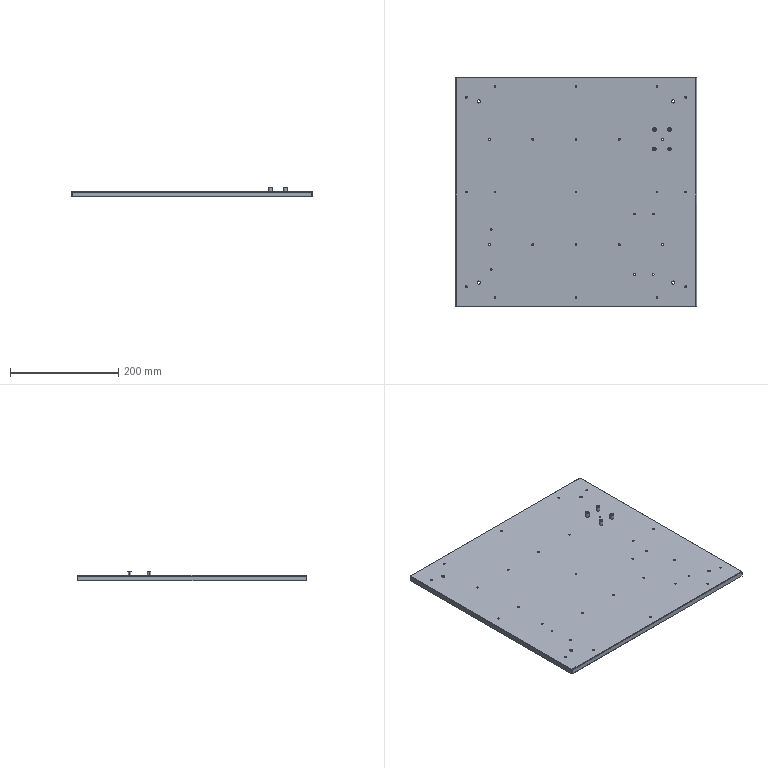Part | STEP file | Control system fixing plate | 1 solid | 144 faces | box 446 x 425 x 18 mm | volume 245891 mm3 | cylinder 94 | plane 26 | cone 16 | spline 8 | commonest cylinder face diameters 3.3 x62 2.5 x8 6 x8 7 x8 0.02 x4 2.42 x4